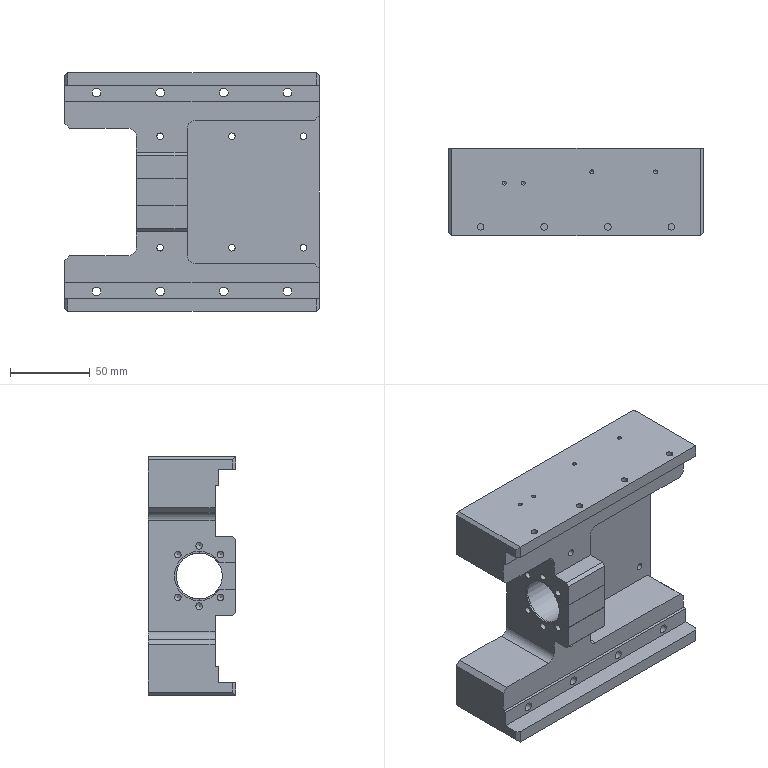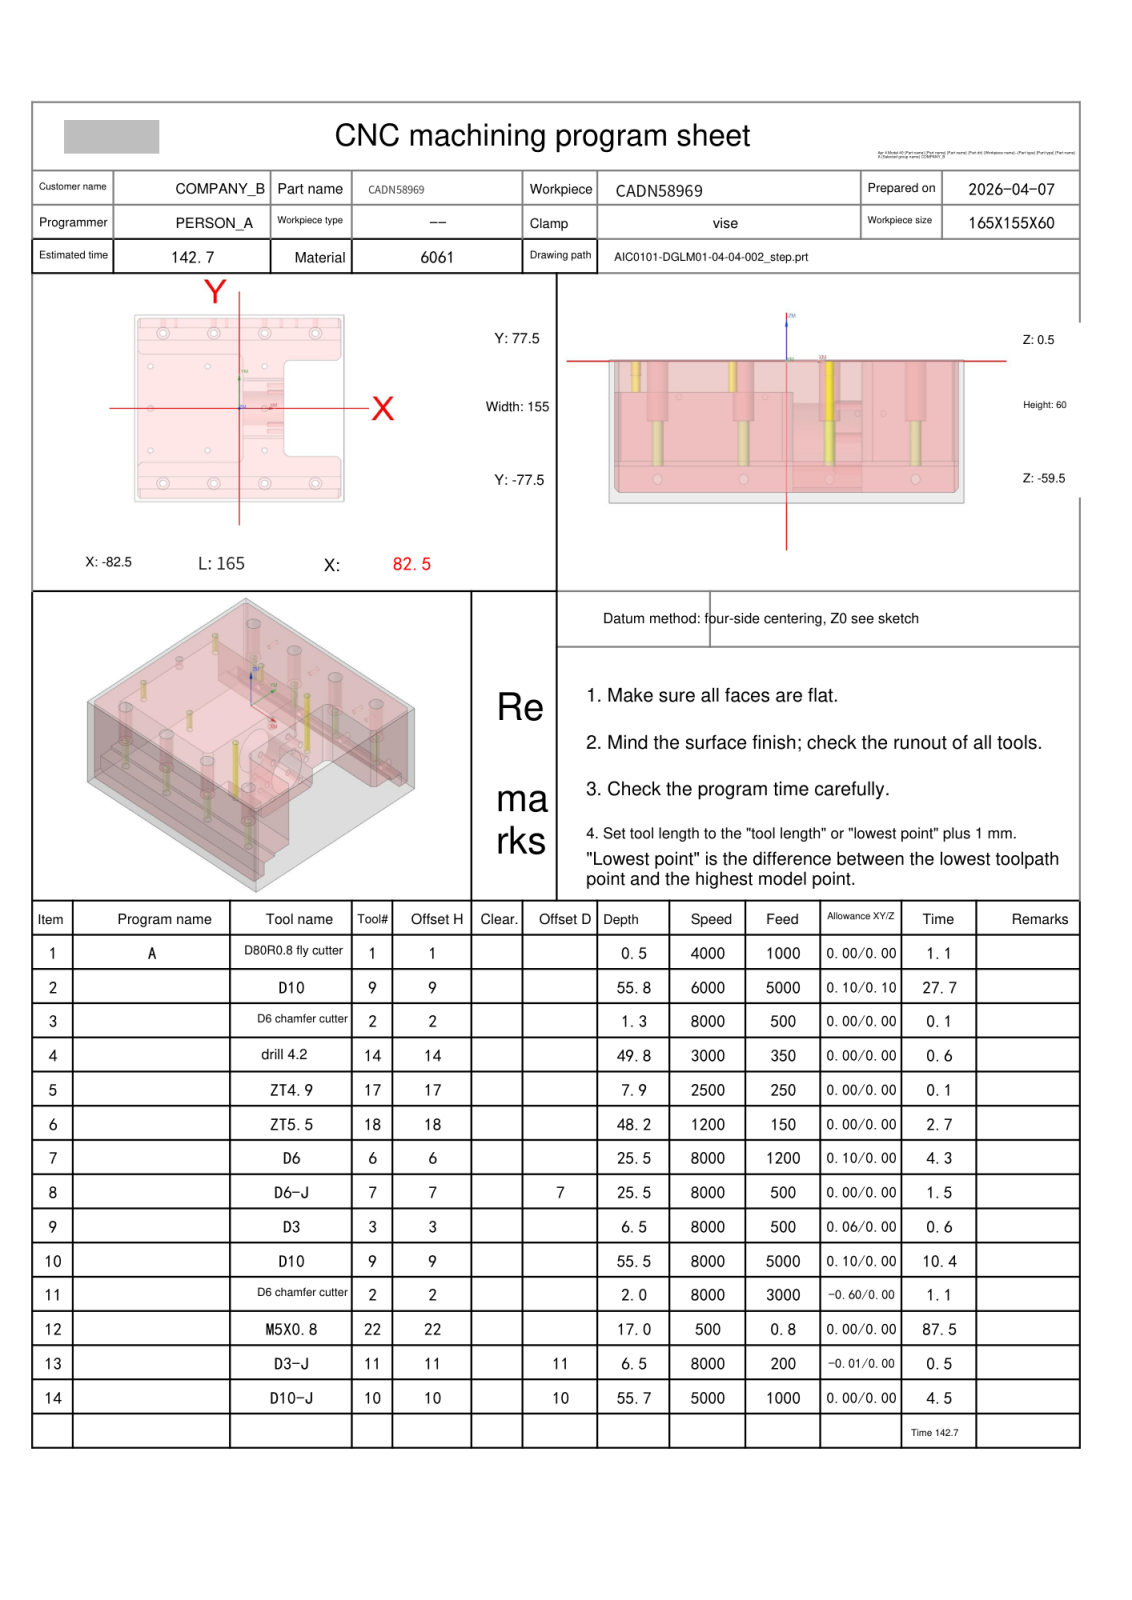NC program | NX | posted by the shop | part box 160 x 55 x 150 mm
Lines 45 to 1090 of 15707:
N2 T09 M06
(D10  D=10. R=0. H=09 ce=0.10 di=0.10)
G00 G90 G54 X94.5 Y.734 M03 S6000
G43 H09 Z10.5
M08
Z.702
G01 Z-.498 F5000.
G02 X89.333 Y-1.543 I-5.167 J4.722
X87.5 Y-1.299 I0.0 J7.
G03 X83.279 Y-.395 I-10.5 J-38.701
G02 X82.944 Y0.0 I.065 J.395
X83.279 Y.395 I.4 J0.0
G03 X86.743 Y1.102 I-6.279 J39.605
X87.5 Y2.071 I-.243 J.97
G01 Y7.652
G03 X86.8 Y8.352 I-.7 J0.0
X86.597 Y8.322 I0.0 J-.7
G02 X77. Y6.9 I-9.597 J31.678
G01 X69.096
G03 X68.1 Y5.904 I.004 J-1.
G01 Y-2.564
X68.078 Y-2.653
X68.156 Y-2.699
X68.29 Y-2.831
G02 X68.377 Y-3.015 I-.21 J-.213
G03 X70.866 Y-5.276 I2.489 J.238
X71.779 Y-5.104 I0.0 J2.5
G01 X81.091 Y-1.451
G03 X82.679 Y.876 I-.913 J2.327
X80.179 Y3.376 I-2.5 J0.0
X79.266 Y3.204 I0.0 J-2.5
G01 X69.953 Y-.449
G03 X68.374 Y-2.575 I.913 J-2.327
G01 X68.393 Y-2.656
X68.318 Y-2.694
X68.191 Y-2.819
G03 X68.1 Y-3.037 I.215 J-.218
G01 Y-5.904
G03 X69.096 Y-6.9 I1. J.004
G01 X77.
G02 X86.796 Y-8.383 I0.0 J-33.1
X87.5 Y-9.338 I-.296 J-.955
G01 Y-15.203
G02 X86.9 Y-15.803 I-.6 J0.0
X86.678 Y-15.761 I0.0 J.6
G03 X77. Y-13.9 I-9.678 J-24.239
G01 X62.097
G02 X61.1 Y-12.903 I.003 J1.
G01 Y12.903
G02 X62.097 Y13.9 I1. J-.003
G01 X77.
G03 X86.879 Y15.842 I0.0 J26.1
X87.5 Y16.767 I-.379 J.925
G01 Y23.143
G03 X87. Y23.643 I-.5 J0.0
X86.745 Y23.573 I0.0 J-.5
G02 X77. Y20.9 I-9.745 J16.427
G01 X55.097
G03 X54.1 Y19.903 I.003 J-1.
G01 Y-19.903
G03 X55.097 Y-20.9 I1. J.003
G01 X77.
G02 X87.025 Y-23.743 I0.0 J-19.1
X87.5 Y-24.593 I-.525 J-.851
G01 Y-32.423
G02 X87.1 Y-32.822 I-.4 J0.0
X86.817 Y-32.705 I0.0 J.4
G01 X85.556 Y-31.444
G03 X77. Y-27.9 I-8.556 J-8.556
G01 X48.098
G02 X47.1 Y-26.902 I.002 J1.
G01 Y26.902
G02 X48.098 Y27.9 I1. J-.002
G01 X77.
G03 X85.556 Y31.444 I0.0 J12.1
G01 X86.903 Y32.791
G03 X87.195 Y33.498 I-.707 J.707
X87.011 Y34.077 I-1. J0.0
G01 X84.072 Y38.21
G03 X83.257 Y38.631 I-.815 J-.579
X82.55 Y38.338 I0.0 J-1.
G01 X80.606 Y36.394
G02 X77. Y34.9 I-3.606 J3.606
G01 X40.1
Y-34.9
X77.
G02 X80.606 Y-36.394 I0.0 J-5.1
G01 X83.606 Y-39.394
G02 X85.1 Y-43. I-3.606 J-3.606
G01 Y-73.001
G02 X83.606 Y-76.606 I-5.1 J.001
G01 X81.606 Y-78.606
G02 X78. Y-80.1 I-3.606 J3.606
G01 X-78.
G02 X-81.606 Y-78.606 I0.0 J5.1
G01 X-83.606 Y-76.606
G02 X-85.1 Y-73.001 I3.606 J3.606
G01 Y73.001
G02 X-83.606 Y76.606 I5.1 J-.001
G01 X-81.606 Y78.606
G02 X-78. Y80.1 I3.606 J-3.606
G01 X78.
G02 X81.606 Y78.606 I0.0 J-5.1
G01 X83.606 Y76.606
G02 X85.1 Y73.001 I-3.606 J-3.606
G01 Y43.
G02 X83.606 Y39.394 I-5.1 J0.0
G01 X80.606 Y36.394
G02 X78.72 Y35.199 I-3.606 J3.606
X78.242 Y35.054 I-1.72 J4.801
G03 X72.947 Y28.264 I1.705 J-6.789
X73.158 Y26.559 I7. J0.0
G01 Z.702
G00 Z3.
G01 X94.5 Y.734 F6000.
G00 Z.204
G01 Z-.996 F5000.
G02 X89.333 Y-1.543 I-5.167 J4.722
X87.5 Y-1.299 I0.0 J7.
G03 X83.279 Y-.395 I-10.5 J-38.701
G02 X82.944 Y0.0 I.065 J.395
X83.279 Y.395 I.4 J0.0
G03 X86.743 Y1.102 I-6.279 J39.605
X87.5 Y2.071 I-.243 J.97
G01 Y7.652
G03 X86.8 Y8.352 I-.7 J0.0
X86.597 Y8.322 I0.0 J-.7
G02 X77. Y6.9 I-9.597 J31.678
G01 X69.096
G03 X68.1 Y5.904 I.004 J-1.
G01 Y2.988
X68.078 Y2.9
X68.156 Y2.854
X68.29 Y2.722
G02 X68.377 Y2.538 I-.21 J-.213
G03 X69.953 Y.449 I2.489 J.238
G01 X79.266 Y-3.204
G03 X80.179 Y-3.376 I.913 J2.327
X82.679 Y-.876 I0.0 J2.5
X81.091 Y1.451 I-2.5 J0.0
G01 X71.779 Y5.104
G03 X70.866 Y5.276 I-.913 J-2.327
X68.374 Y2.978 I0.0 J-2.5
G01 X68.393 Y2.897
X68.318 Y2.859
X68.191 Y2.734
G03 X68.1 Y2.515 I.215 J-.218
G01 Y-5.904
G03 X69.096 Y-6.9 I1. J.004
G01 X77.
G02 X86.796 Y-8.383 I0.0 J-33.1
X87.5 Y-9.338 I-.296 J-.955
G01 Y-15.203
G02 X86.9 Y-15.803 I-.6 J0.0
X86.678 Y-15.761 I0.0 J.6
G03 X77. Y-13.9 I-9.678 J-24.239
G01 X62.097
G02 X61.1 Y-12.903 I.003 J1.
G01 Y12.903
G02 X62.097 Y13.9 I1. J-.003
G01 X77.
G03 X86.879 Y15.842 I0.0 J26.1
X87.5 Y16.767 I-.379 J.925
G01 Y23.143
G03 X87. Y23.643 I-.5 J0.0
X86.745 Y23.573 I0.0 J-.5
G02 X77. Y20.9 I-9.745 J16.427
G01 X55.097
G03 X54.1 Y19.903 I.003 J-1.
G01 Y-19.903
G03 X55.097 Y-20.9 I1. J.003
G01 X77.
G02 X87.025 Y-23.742 I0.0 J-19.1
X87.5 Y-24.593 I-.525 J-.851
G01 Y-32.423
G02 X87.1 Y-32.822 I-.4 J0.0
X86.817 Y-32.705 I0.0 J.4
G01 X85.556 Y-31.444
G03 X77. Y-27.9 I-8.556 J-8.556
G01 X48.098
G02 X47.1 Y-26.902 I.002 J1.
G01 Y26.902
G02 X48.098 Y27.9 I1. J-.002
G01 X77.
G03 X85.556 Y31.444 I0.0 J12.1
G01 X86.903 Y32.791
G03 X87.195 Y33.498 I-.707 J.707
X87.011 Y34.077 I-1. J0.0
G01 X84.072 Y38.21
G03 X83.257 Y38.631 I-.815 J-.579
X82.55 Y38.338 I0.0 J-1.
G01 X80.606 Y36.394
G02 X77. Y34.9 I-3.606 J3.606
G01 X40.1
Y-34.9
X77.
G02 X80.606 Y-36.394 I0.0 J-5.1
G01 X83.606 Y-39.394
G02 X85.1 Y-43. I-3.606 J-3.606
G01 Y-73.001
G02 X83.606 Y-76.606 I-5.1 J.001
G01 X81.606 Y-78.606
G02 X78. Y-80.1 I-3.606 J3.606
G01 X-78.
G02 X-81.606 Y-78.606 I0.0 J5.1
G01 X-83.606 Y-76.606
G02 X-85.1 Y-73.001 I3.606 J3.606
G01 Y73.001
G02 X-83.606 Y76.606 I5.1 J-.001
G01 X-81.606 Y78.606
G02 X-78. Y80.1 I3.606 J-3.606
G01 X78.
G02 X81.606 Y78.606 I0.0 J-5.1
G01 X83.606 Y76.606
G02 X85.1 Y73.001 I-3.606 J-3.606
G01 Y43.
G02 X83.606 Y39.394 I-5.1 J0.0
G01 X80.606 Y36.394
G02 X78.72 Y35.199 I-3.606 J3.606
X78.242 Y35.054 I-1.72 J4.801
G03 X72.947 Y28.264 I1.705 J-6.789
X73.158 Y26.559 I7. J0.0
G01 Z.204
G00 Z2.502
G01 X94.5 Y.734 F6000.
G00 Z-.295
G01 Z-1.495 F5000.
G02 X89.333 Y-1.543 I-5.167 J4.722
X87.5 Y-1.299 I0.0 J7.
G03 X83.279 Y-.395 I-10.5 J-38.701
G02 X82.944 Y0.0 I.065 J.395
X83.279 Y.395 I.4 J0.0
G03 X86.743 Y1.102 I-6.279 J39.605
X87.5 Y2.071 I-.243 J.97
G01 Y7.652
G03 X86.8 Y8.352 I-.7 J0.0
X86.597 Y8.322 I0.0 J-.7
G02 X77. Y6.9 I-9.597 J31.678
G01 X69.097
G03 X68.1 Y5.903 I.003 J-1.
G01 Y2.988
X68.078 Y2.9
X68.156 Y2.854
X68.29 Y2.722
G02 X68.377 Y2.538 I-.21 J-.213
G03 X69.953 Y.449 I2.489 J.238
G01 X79.266 Y-3.204
G03 X80.179 Y-3.376 I.913 J2.327
X82.679 Y-.876 I0.0 J2.5
X81.091 Y1.451 I-2.5 J0.0
G01 X71.779 Y5.104
G03 X70.866 Y5.276 I-.913 J-2.327
X68.374 Y2.978 I0.0 J-2.5
G01 X68.393 Y2.897
X68.318 Y2.859
X68.191 Y2.734
G03 X68.1 Y2.515 I.215 J-.218
G01 Y-5.903
G03 X69.097 Y-6.9 I1. J.003
G01 X77.
G02 X86.796 Y-8.383 I0.0 J-33.1
X87.5 Y-9.338 I-.296 J-.955
G01 Y-15.203
G02 X86.9 Y-15.803 I-.6 J0.0
X86.678 Y-15.761 I0.0 J.6
G03 X77. Y-13.9 I-9.678 J-24.239
G01 X62.097
G02 X61.1 Y-12.903 I.003 J1.
G01 Y12.903
G02 X62.097 Y13.9 I1. J-.003
G01 X77.
G03 X86.879 Y15.842 I0.0 J26.1
X87.5 Y16.767 I-.379 J.925
G01 Y23.143
G03 X87. Y23.643 I-.5 J0.0
X86.745 Y23.573 I0.0 J-.5
G02 X77. Y20.9 I-9.745 J16.427
G01 X55.098
G03 X54.1 Y19.902 I.002 J-1.
G01 Y-19.902
G03 X55.098 Y-20.9 I1. J.002
G01 X77.
G02 X87.025 Y-23.743 I0.0 J-19.1
X87.5 Y-24.593 I-.525 J-.851
G01 Y-32.423
G02 X87.1 Y-32.822 I-.4 J0.0
X86.817 Y-32.705 I0.0 J.4
G01 X85.556 Y-31.444
G03 X77. Y-27.9 I-8.556 J-8.556
G01 X48.099
G02 X47.1 Y-26.901 I.001 J1.
G01 Y26.901
G02 X48.099 Y27.9 I1. J-.001
G01 X77.
G03 X85.556 Y31.444 I0.0 J12.1
G01 X86.903 Y32.791
G03 X87.195 Y33.498 I-.707 J.707
X87.011 Y34.077 I-1. J0.0
G01 X84.072 Y38.21
G03 X83.257 Y38.631 I-.815 J-.579
X82.55 Y38.338 I0.0 J-1.
G01 X80.606 Y36.394
G02 X77. Y34.9 I-3.606 J3.606
G01 X40.1
Y-34.9
X77.
G02 X80.606 Y-36.394 I0.0 J-5.1
G01 X83.606 Y-39.394
G02 X85.1 Y-43. I-3.606 J-3.606
G01 Y-73.
G02 X83.606 Y-76.606 I-5.1 J0.0
G01 X81.606 Y-78.606
G02 X78. Y-80.1 I-3.606 J3.606
G01 X-78.
G02 X-81.606 Y-78.606 I0.0 J5.1
G01 X-83.606 Y-76.606
G02 X-85.1 Y-73. I3.606 J3.606
G01 Y73.
G02 X-83.606 Y76.606 I5.1 J0.0
G01 X-81.606 Y78.606
G02 X-78. Y80.1 I3.606 J-3.606
G01 X78.
G02 X81.606 Y78.606 I0.0 J-5.1
G01 X83.606 Y76.606
G02 X85.1 Y73. I-3.606 J-3.606
G01 Y43.
G02 X83.606 Y39.394 I-5.1 J0.0
G01 X80.606 Y36.394
G02 X78.72 Y35.199 I-3.606 J3.606
X78.242 Y35.054 I-1.72 J4.801
G03 X72.947 Y28.264 I1.705 J-6.789
X73.158 Y26.559 I7. J0.0
G01 Z-.295
G00 Z2.004
G01 X94.5 Y.734 F6000.
G00 Z-.793
G01 Z-1.993 F5000.
G02 X89.333 Y-1.543 I-5.167 J4.722
X87.5 Y-1.299 I0.0 J7.
G03 X83.279 Y-.395 I-10.5 J-38.701
G02 X82.944 Y0.0 I.065 J.395
X83.279 Y.395 I.4 J0.0
G03 X86.743 Y1.102 I-6.279 J39.605
X87.5 Y2.071 I-.243 J.97
G01 Y7.652
G03 X86.8 Y8.352 I-.7 J0.0
X86.597 Y8.322 I0.0 J-.7
G02 X77. Y6.9 I-9.597 J31.678
G01 X69.096
G03 X68.1 Y5.904 I.004 J-1.
G01 Y-2.564
X68.078 Y-2.653
X68.156 Y-2.699
X68.29 Y-2.831
G02 X68.377 Y-3.015 I-.21 J-.213
G03 X70.866 Y-5.276 I2.489 J.238
X71.779 Y-5.104 I0.0 J2.5
G01 X81.091 Y-1.451
G03 X82.679 Y.876 I-.913 J2.327
X80.179 Y3.376 I-2.5 J0.0
X79.266 Y3.204 I0.0 J-2.5
G01 X69.953 Y-.449
G03 X68.374 Y-2.575 I.913 J-2.327
G01 X68.393 Y-2.656
X68.318 Y-2.694
X68.191 Y-2.819
G03 X68.1 Y-3.037 I.215 J-.218
G01 Y-5.904
G03 X69.096 Y-6.9 I1. J.004
G01 X77.
G02 X86.796 Y-8.383 I0.0 J-33.1
X87.5 Y-9.338 I-.296 J-.955
G01 Y-15.203
G02 X86.9 Y-15.803 I-.6 J0.0
X86.678 Y-15.761 I0.0 J.6
G03 X77. Y-13.9 I-9.678 J-24.239
G01 X62.097
G02 X61.1 Y-12.903 I.003 J1.
G01 Y12.903
G02 X62.097 Y13.9 I1. J-.003
G01 X77.
G03 X86.879 Y15.842 I0.0 J26.1
X87.5 Y16.767 I-.379 J.925
G01 Y23.143
G03 X87. Y23.643 I-.5 J0.0
X86.745 Y23.573 I0.0 J-.5
G02 X77. Y20.9 I-9.745 J16.427
G01 X55.098
G03 X54.1 Y19.902 I.002 J-1.
G01 Y-19.902
G03 X55.098 Y-20.9 I1. J.002
G01 X77.
G02 X87.025 Y-23.743 I0.0 J-19.1
X87.5 Y-24.593 I-.525 J-.851
G01 Y-32.423
G02 X87.1 Y-32.822 I-.4 J0.0
X86.817 Y-32.705 I0.0 J.4
G01 X85.556 Y-31.444
G03 X77. Y-27.9 I-8.556 J-8.556
G01 X48.099
G02 X47.1 Y-26.901 I.001 J1.
G01 Y26.901
G02 X48.099 Y27.9 I1. J-.001
G01 X77.
G03 X85.556 Y31.444 I0.0 J12.1
G01 X86.903 Y32.791
G03 X87.195 Y33.498 I-.707 J.707
X87.011 Y34.077 I-1. J0.0
G01 X84.072 Y38.21
G03 X83.257 Y38.631 I-.815 J-.579
X82.55 Y38.338 I0.0 J-1.
G01 X80.606 Y36.394
G02 X77. Y34.9 I-3.606 J3.606
G01 X40.1
Y-34.9
X77.
G02 X80.606 Y-36.394 I0.0 J-5.1
G01 X83.606 Y-39.394
G02 X85.1 Y-43. I-3.606 J-3.606
G01 Y-73.
G02 X83.606 Y-76.606 I-5.1 J0.0
G01 X81.606 Y-78.606
G02 X78. Y-80.1 I-3.606 J3.606
G01 X-78.
G02 X-81.606 Y-78.606 I0.0 J5.1
G01 X-83.606 Y-76.606
G02 X-85.1 Y-73. I3.606 J3.606
G01 Y73.
G02 X-83.606 Y76.606 I5.1 J0.0
G01 X-81.606 Y78.606
G02 X-78. Y80.1 I3.606 J-3.606
G01 X78.
G02 X81.606 Y78.606 I0.0 J-5.1
G01 X83.606 Y76.606
G02 X85.1 Y73. I-3.606 J-3.606
G01 Y43.
G02 X83.606 Y39.394 I-5.1 J0.0
G01 X80.606 Y36.394
G02 X78.72 Y35.199 I-3.606 J3.606
X78.242 Y35.054 I-1.72 J4.801
G03 X72.947 Y28.264 I1.705 J-6.789
X73.158 Y26.559 I7. J0.0
G01 Z-.793
G00 Z1.505
G01 X94.5 Y.734 F6000.
G00 Z-1.291
G01 Z-2.491 F5000.
G02 X89.333 Y-1.543 I-5.167 J4.722
X87.5 Y-1.299 I0.0 J7.
G03 X83.279 Y-.395 I-10.5 J-38.701
G02 X82.944 Y0.0 I.065 J.395
X83.279 Y.395 I.4 J0.0
G03 X86.743 Y1.102 I-6.279 J39.605
X87.5 Y2.071 I-.243 J.97
G01 Y7.652
G03 X86.8 Y8.352 I-.7 J0.0
X86.597 Y8.322 I0.0 J-.7
G02 X77. Y6.9 I-9.597 J31.678
G01 X69.097
G03 X68.1 Y5.903 I.003 J-1.
G01 Y2.988
X68.078 Y2.9
X68.156 Y2.854
X68.29 Y2.722
G02 X68.377 Y2.538 I-.21 J-.213
G03 X69.953 Y.449 I2.489 J.238
G01 X79.266 Y-3.204
G03 X80.179 Y-3.376 I.913 J2.327
X82.679 Y-.876 I0.0 J2.5
X81.091 Y1.451 I-2.5 J0.0
G01 X71.779 Y5.104
G03 X70.866 Y5.276 I-.913 J-2.327
X68.374 Y2.978 I0.0 J-2.5
G01 X68.393 Y2.897
X68.318 Y2.859
X68.191 Y2.734
G03 X68.1 Y2.515 I.215 J-.218
G01 Y-5.903
G03 X69.097 Y-6.9 I1. J.003
G01 X77.
G02 X86.796 Y-8.383 I0.0 J-33.1
X87.5 Y-9.338 I-.296 J-.955
G01 Y-15.203
G02 X86.9 Y-15.803 I-.6 J0.0
X86.678 Y-15.761 I0.0 J.6
G03 X77. Y-13.9 I-9.678 J-24.239
G01 X62.097
G02 X61.1 Y-12.903 I.003 J1.
G01 Y12.903
G02 X62.097 Y13.9 I1. J-.003
G01 X77.
G03 X86.879 Y15.842 I0.0 J26.1
X87.5 Y16.767 I-.379 J.925
G01 Y23.143
G03 X87. Y23.643 I-.5 J0.0
X86.745 Y23.573 I0.0 J-.5
G02 X77. Y20.9 I-9.745 J16.427
G01 X55.098
G03 X54.1 Y19.902 I.002 J-1.
G01 Y-19.902
G03 X55.098 Y-20.9 I1. J.002
G01 X77.
G02 X87.025 Y-23.743 I0.0 J-19.1
X87.5 Y-24.593 I-.525 J-.851
G01 Y-32.423
G02 X87.1 Y-32.822 I-.4 J0.0
X86.817 Y-32.705 I0.0 J.4
G01 X85.556 Y-31.444
G03 X77. Y-27.9 I-8.556 J-8.556
G01 X48.099
G02 X47.1 Y-26.901 I.001 J1.
G01 Y26.901
G02 X48.099 Y27.9 I1. J-.001
G01 X77.
G03 X85.556 Y31.444 I0.0 J12.1
G01 X86.903 Y32.791
G03 X87.195 Y33.498 I-.707 J.707
X87.011 Y34.077 I-1. J0.0
G01 X84.072 Y38.21
G03 X83.257 Y38.631 I-.815 J-.579
X82.55 Y38.338 I0.0 J-1.
G01 X80.606 Y36.394
G02 X77. Y34.9 I-3.606 J3.606
G01 X40.1
Y-34.9
X77.
G02 X80.606 Y-36.394 I0.0 J-5.1
G01 X83.606 Y-39.394
G02 X85.1 Y-43. I-3.606 J-3.606
G01 Y-73.
G02 X83.606 Y-76.606 I-5.1 J0.0
G01 X81.606 Y-78.606
G02 X78. Y-80.1 I-3.606 J3.606
G01 X-78.
G02 X-81.606 Y-78.606 I0.0 J5.1
G01 X-83.606 Y-76.606
G02 X-85.1 Y-73. I3.606 J3.606
G01 Y73.
G02 X-83.606 Y76.606 I5.1 J0.0
G01 X-81.606 Y78.606
G02 X-78. Y80.1 I3.606 J-3.606
G01 X78.
G02 X81.606 Y78.606 I0.0 J-5.1
G01 X83.606 Y76.606
G02 X85.1 Y73. I-3.606 J-3.606
G01 Y43.
G02 X83.606 Y39.394 I-5.1 J0.0
G01 X80.606 Y36.394
G02 X78.72 Y35.199 I-3.606 J3.606
X78.242 Y35.054 I-1.72 J4.801
G03 X72.947 Y28.264 I1.705 J-6.789
X73.158 Y26.559 I7. J0.0
G01 Z-1.291
G00 Z1.007
G01 X94.5 Y.734 F6000.
G00 Z-1.789
G01 Z-2.989 F5000.
G02 X89.333 Y-1.543 I-5.167 J4.722
X87.5 Y-1.299 I0.0 J7.
G03 X83.279 Y-.395 I-10.5 J-38.701
G02 X82.944 Y0.0 I.065 J.395
X83.279 Y.395 I.4 J0.0
G03 X86.743 Y1.102 I-6.279 J39.605
X87.5 Y2.071 I-.243 J.97
G01 Y7.652
G03 X86.8 Y8.352 I-.7 J0.0
X86.597 Y8.322 I0.0 J-.7
G02 X77. Y6.9 I-9.597 J31.678
G01 X69.096
G03 X68.1 Y5.904 I.004 J-1.
G01 Y-2.564
X68.078 Y-2.653
X68.156 Y-2.699
X68.29 Y-2.831
G02 X68.377 Y-3.015 I-.21 J-.213
G03 X70.866 Y-5.276 I2.489 J.238
X71.779 Y-5.104 I0.0 J2.5
G01 X81.091 Y-1.451
G03 X82.679 Y.876 I-.913 J2.327
X80.179 Y3.376 I-2.5 J0.0
X79.266 Y3.204 I0.0 J-2.5
G01 X69.953 Y-.449
G03 X68.374 Y-2.575 I.913 J-2.327
G01 X68.393 Y-2.656
X68.318 Y-2.694
X68.191 Y-2.819
G03 X68.1 Y-3.037 I.215 J-.218
G01 Y-5.904
G03 X69.096 Y-6.9 I1. J.004
G01 X77.
G02 X86.796 Y-8.383 I0.0 J-33.1
X87.5 Y-9.338 I-.296 J-.955
G01 Y-15.203
G02 X86.9 Y-15.803 I-.6 J0.0
X86.678 Y-15.761 I0.0 J.6
G03 X77. Y-13.9 I-9.678 J-24.239
G01 X62.097
G02 X61.1 Y-12.903 I.003 J1.
G01 Y12.903
G02 X62.097 Y13.9 I1. J-.003
G01 X77.
G03 X86.879 Y15.842 I0.0 J26.1
X87.5 Y16.767 I-.379 J.925
G01 Y23.143
G03 X87. Y23.643 I-.5 J0.0
X86.745 Y23.573 I0.0 J-.5
G02 X77. Y20.9 I-9.745 J16.427
G01 X55.098
G03 X54.1 Y19.902 I.002 J-1.
G01 Y-19.902
G03 X55.098 Y-20.9 I1. J.002
G01 X77.
G02 X87.025 Y-23.743 I0.0 J-19.1
X87.5 Y-24.593 I-.525 J-.851
G01 Y-32.423
G02 X87.1 Y-32.822 I-.4 J0.0
X86.817 Y-32.705 I0.0 J.4
G01 X85.556 Y-31.444
G03 X77. Y-27.9 I-8.556 J-8.556
G01 X48.099
G02 X47.1 Y-26.901 I.001 J1.
G01 Y26.901
G02 X48.099 Y27.9 I1. J-.001
G01 X77.
G03 X85.556 Y31.444 I0.0 J12.1
G01 X86.903 Y32.791
G03 X87.195 Y33.498 I-.707 J.707
X87.011 Y34.077 I-1. J0.0
G01 X84.072 Y38.21
G03 X83.257 Y38.631 I-.815 J-.579
X82.55 Y38.338 I0.0 J-1.
G01 X80.606 Y36.394
G02 X77. Y34.9 I-3.606 J3.606
G01 X40.1
Y-34.9
X77.
G02 X80.606 Y-36.394 I0.0 J-5.1
G01 X83.606 Y-39.394
G02 X85.1 Y-43. I-3.606 J-3.606
G01 Y-73.
G02 X83.606 Y-76.606 I-5.1 J0.0
G01 X81.606 Y-78.606
G02 X78. Y-80.1 I-3.606 J3.606
G01 X-78.
G02 X-81.606 Y-78.606 I0.0 J5.1
G01 X-83.606 Y-76.606
G02 X-85.1 Y-73. I3.606 J3.606
G01 Y73.
G02 X-83.606 Y76.606 I5.1 J0.0
G01 X-81.606 Y78.606
G02 X-78. Y80.1 I3.606 J-3.606
G01 X78.
G02 X81.606 Y78.606 I0.0 J-5.1
G01 X83.606 Y76.606
G02 X85.1 Y73. I-3.606 J-3.606
G01 Y43.
G02 X83.606 Y39.394 I-5.1 J0.0
G01 X80.606 Y36.394
G02 X78.72 Y35.199 I-3.606 J3.606
X78.242 Y35.054 I-1.72 J4.801
G03 X72.947 Y28.264 I1.705 J-6.789
X73.158 Y26.559 I7. J0.0
G01 Z-1.789
G00 Z.509
G01 X94.5 Y.734 F6000.
G00 Z-2.287
G01 Z-3.487 F5000.
G02 X89.333 Y-1.543 I-5.167 J4.722
X87.5 Y-1.299 I0.0 J7.
G03 X83.279 Y-.395 I-10.5 J-38.701
G02 X82.944 Y0.0 I.065 J.395
X83.279 Y.395 I.4 J0.0
G03 X86.743 Y1.102 I-6.279 J39.605
X87.5 Y2.071 I-.243 J.97
G01 Y7.652
G03 X86.8 Y8.352 I-.7 J0.0
X86.597 Y8.322 I0.0 J-.7
G02 X77. Y6.9 I-9.597 J31.678
G01 X69.097
G03 X68.1 Y5.903 I.003 J-1.
G01 Y2.988
X68.078 Y2.9
X68.156 Y2.854
X68.29 Y2.722
G02 X68.377 Y2.538 I-.21 J-.213
G03 X69.953 Y.449 I2.489 J.238
G01 X79.266 Y-3.204
G03 X80.179 Y-3.376 I.913 J2.327
X82.679 Y-.876 I0.0 J2.5
X81.091 Y1.451 I-2.5 J0.0
G01 X71.779 Y5.104
G03 X70.866 Y5.276 I-.913 J-2.327
X68.374 Y2.978 I0.0 J-2.5
G01 X68.393 Y2.897
X68.318 Y2.859
X68.191 Y2.734
G03 X68.1 Y2.515 I.215 J-.218
G01 Y-5.903
G03 X69.097 Y-6.9 I1. J.003
G01 X77.
G02 X86.796 Y-8.383 I0.0 J-33.1
X87.5 Y-9.338 I-.296 J-.955
G01 Y-15.203
G02 X86.9 Y-15.803 I-.6 J0.0
X86.678 Y-15.761 I0.0 J.6
G03 X77. Y-13.9 I-9.678 J-24.239
G01 X62.097
G02 X61.1 Y-12.903 I.003 J1.
G01 Y12.903
G02 X62.097 Y13.9 I1. J-.003
G01 X77.
G03 X86.879 Y15.842 I0.0 J26.1
X87.5 Y16.767 I-.379 J.925
G01 Y23.143
G03 X87. Y23.643 I-.5 J0.0
X86.745 Y23.573 I0.0 J-.5
G02 X77. Y20.9 I-9.745 J16.427
G01 X55.098
G03 X54.1 Y19.902 I.002 J-1.
G01 Y-19.902
G03 X55.098 Y-20.9 I1. J.002
G01 X77.
G02 X87.025 Y-23.743 I0.0 J-19.1
X87.5 Y-24.593 I-.525 J-.851
G01 Y-32.423
G02 X87.1 Y-32.822 I-.4 J0.0
X86.817 Y-32.705 I0.0 J.4
G01 X85.556 Y-31.444
G03 X77. Y-27.9 I-8.556 J-8.556
G01 X48.099
G02 X47.1 Y-26.901 I.001 J1.
G01 Y26.901
G02 X48.099 Y27.9 I1. J-.001
G01 X77.
G03 X85.556 Y31.444 I0.0 J12.1
G01 X86.903 Y32.791
G03 X87.195 Y33.498 I-.707 J.707
X87.011 Y34.077 I-1. J0.0
G01 X84.072 Y38.21
G03 X83.257 Y38.631 I-.815 J-.579
X82.55 Y38.338 I0.0 J-1.
G01 X80.606 Y36.394
G02 X77. Y34.9 I-3.606 J3.606
G01 X40.1
Y-34.9
X77.
G02 X80.606 Y-36.394 I0.0 J-5.1
G01 X83.606 Y-39.394
G02 X85.1 Y-43. I-3.606 J-3.606
G01 Y-73.
G02 X83.606 Y-76.606 I-5.1 J0.0
G01 X81.606 Y-78.606
G02 X78. Y-80.1 I-3.606 J3.606
G01 X-78.
G02 X-81.606 Y-78.606 I0.0 J5.1
G01 X-83.606 Y-76.606
G02 X-85.1 Y-73. I3.606 J3.606
G01 Y73.
G02 X-83.606 Y76.606 I5.1 J0.0
G01 X-81.606 Y78.606
G02 X-78. Y80.1 I3.606 J-3.606
G01 X78.
G02 X81.606 Y78.606 I0.0 J-5.1
G01 X83.606 Y76.606
G02 X85.1 Y73. I-3.606 J-3.606
G01 Y43.
G02 X83.606 Y39.394 I-5.1 J0.0
G01 X80.606 Y36.394
G02 X78.72 Y35.199 I-3.606 J3.606
X78.242 Y35.054 I-1.72 J4.801
G03 X72.947 Y28.264 I1.705 J-6.789
X73.158 Y26.559 I7. J0.0
G01 Z-2.287
G00 Z.011
G01 X94.5 Y.734 F6000.
G00 Z-2.786
G01 Z-3.986 F5000.
G02 X89.333 Y-1.543 I-5.167 J4.722
X87.5 Y-1.299 I0.0 J7.
G03 X83.279 Y-.395 I-10.5 J-38.701
G02 X82.944 Y0.0 I.065 J.395
X83.279 Y.395 I.4 J0.0
G03 X86.743 Y1.102 I-6.279 J39.605
X87.5 Y2.071 I-.243 J.97
G01 Y7.652
G03 X86.8 Y8.352 I-.7 J0.0
X86.597 Y8.322 I0.0 J-.7
G02 X77. Y6.9 I-9.597 J31.678
G01 X69.096
G03 X68.1 Y5.904 I.004 J-1.
G01 Y-2.564
X68.078 Y-2.653
X68.156 Y-2.699
X68.29 Y-2.831
G02 X68.377 Y-3.015 I-.21 J-.213
G03 X70.866 Y-5.276 I2.489 J.238
X71.779 Y-5.104 I0.0 J2.5
G01 X81.091 Y-1.451
G03 X82.679 Y.876 I-.913 J2.327
X80.179 Y3.376 I-2.5 J0.0
X79.266 Y3.204 I0.0 J-2.5
G01 X69.953 Y-.449
G03 X68.374 Y-2.575 I.913 J-2.327
G01 X68.393 Y-2.656
X68.318 Y-2.694
X68.191 Y-2.819
G03 X68.1 Y-3.037 I.215 J-.218
G01 Y-5.904
G03 X69.096 Y-6.9 I1. J.004
G01 X77.
G02 X86.796 Y-8.383 I0.0 J-33.1
X87.5 Y-9.338 I-.296 J-.955
G01 Y-15.203
G02 X86.9 Y-15.803 I-.6 J0.0
X86.678 Y-15.761 I0.0 J.6
G03 X77. Y-13.9 I-9.678 J-24.239
G01 X62.097
G02 X61.1 Y-12.903 I.003 J1.
G01 Y12.903
G02 X62.097 Y13.9 I1. J-.003
G01 X77.
G03 X86.879 Y15.842 I0.0 J26.1
X87.5 Y16.767 I-.379 J.925
G01 Y23.143
G03 X87. Y23.643 I-.5 J0.0
X86.745 Y23.573 I0.0 J-.5
G02 X77. Y20.9 I-9.745 J16.427
G01 X55.098
G03 X54.1 Y19.902 I.002 J-1.
G01 Y-19.902
G03 X55.098 Y-20.9 I1. J.002
G01 X77.
G02 X87.025 Y-23.743 I0.0 J-19.1
X87.5 Y-24.593 I-.525 J-.851
G01 Y-32.423
G02 X87.1 Y-32.822 I-.4 J0.0
X86.817 Y-32.705 I0.0 J.4
G01 X85.556 Y-31.444
G03 X77. Y-27.9 I-8.556 J-8.556
G01 X48.099
G02 X47.1 Y-26.901 I.001 J1.
G01 Y26.901
G02 X48.099 Y27.9 I1. J-.001
G01 X77.
G03 X85.556 Y31.444 I0.0 J12.1
G01 X86.903 Y32.791
G03 X87.195 Y33.498 I-.707 J.707
X87.011 Y34.077 I-1. J0.0
G01 X84.072 Y38.21
G03 X83.257 Y38.631 I-.815 J-.579
X82.55 Y38.338 I0.0 J-1.
G01 X80.606 Y36.394
G02 X77. Y34.9 I-3.606 J3.606
G01 X40.1
Y-34.9
X77.
G02 X80.606 Y-36.394 I0.0 J-5.1
G01 X83.606 Y-39.394
G02 X85.1 Y-43. I-3.606 J-3.606
G01 Y-73.
G02 X83.606 Y-76.606 I-5.1 J0.0
G01 X81.606 Y-78.606
G02 X78. Y-80.1 I-3.606 J3.606
G01 X-78.
G02 X-81.606 Y-78.606 I0.0 J5.1
G01 X-83.606 Y-76.606
G02 X-85.1 Y-73. I3.606 J3.606
G01 Y73.
G02 X-83.606 Y76.606 I5.1 J0.0
G01 X-81.606 Y78.606
G02 X-78. Y80.1 I3.606 J-3.606
G01 X78.
G02 X81.606 Y78.606 I0.0 J-5.1
G01 X83.606 Y76.606
G02 X85.1 Y73. I-3.606 J-3.606
G01 Y43.
G02 X83.606 Y39.394 I-5.1 J0.0
G01 X80.606 Y36.394
G02 X78.72 Y35.199 I-3.606 J3.606
X78.242 Y35.054 I-1.72 J4.801
G03 X72.947 Y28.264 I1.705 J-6.789
X73.158 Y26.559 I7. J0.0
G01 Z-2.786
G00 Z-.487
G01 X94.5 Y.734 F6000.
G00 Z-3.284
G01 Z-4.484 F5000.
G02 X89.333 Y-1.543 I-5.167 J4.722
X87.5 Y-1.299 I0.0 J7.
G03 X83.279 Y-.395 I-10.5 J-38.701
G02 X82.944 Y0.0 I.065 J.395
X83.279 Y.395 I.4 J0.0
G03 X86.743 Y1.102 I-6.279 J39.605
X87.5 Y2.071 I-.243 J.97
G01 Y7.652
G03 X86.8 Y8.352 I-.7 J0.0
X86.597 Y8.322 I0.0 J-.7
G02 X77. Y6.9 I-9.597 J31.678
G01 X69.097
G03 X68.1 Y5.903 I.003 J-1.
G01 Y2.988
X68.078 Y2.9
X68.156 Y2.854
X68.29 Y2.722
G02 X68.377 Y2.538 I-.21 J-.213
G03 X69.953 Y.449 I2.489 J.238
G01 X79.266 Y-3.204
G03 X80.179 Y-3.376 I.913 J2.327
X82.679 Y-.876 I0.0 J2.5
X81.091 Y1.451 I-2.5 J0.0
G01 X71.779 Y5.104
G03 X70.866 Y5.276 I-.913 J-2.327
X68.374 Y2.978 I0.0 J-2.5
G01 X68.393 Y2.897
X68.318 Y2.859
X68.191 Y2.734
G03 X68.1 Y2.515 I.215 J-.218
G01 Y-5.903
G03 X69.097 Y-6.9 I1. J.003
G01 X77.
G02 X86.796 Y-8.383 I0.0 J-33.1
X87.5 Y-9.338 I-.296 J-.955
G01 Y-15.203
G02 X86.9 Y-15.803 I-.6 J0.0
X86.678 Y-15.761 I0.0 J.6
G03 X77. Y-13.9 I-9.678 J-24.239
G01 X62.097
G02 X61.1 Y-12.903 I.003 J1.
G01 Y12.903
G02 X62.097 Y13.9 I1. J-.003
G01 X77.
G03 X86.879 Y15.842 I0.0 J26.1
X87.5 Y16.767 I-.379 J.925
G01 Y23.143
G03 X87. Y23.643 I-.5 J0.0
X86.745 Y23.573 I0.0 J-.5
G02 X77. Y20.9 I-9.745 J16.427
G01 X55.098
G03 X54.1 Y19.902 I.002 J-1.
G01 Y-19.902
G03 X55.098 Y-20.9 I1. J.002
G01 X77.
G02 X87.025 Y-23.743 I0.0 J-19.1
X87.5 Y-24.593 I-.525 J-.851
G01 Y-32.423
G02 X87.1 Y-32.822 I-.4 J0.0
X86.817 Y-32.705 I0.0 J.4
G01 X85.556 Y-31.444
G03 X77. Y-27.9 I-8.556 J-8.556
G01 X48.099
G02 X47.1 Y-26.901 I.001 J1.
G01 Y26.901
G02 X48.099 Y27.9 I1. J-.001
G01 X77.
G03 X85.556 Y31.444 I0.0 J12.1
G01 X86.903 Y32.791
G03 X87.195 Y33.498 I-.707 J.707
X87.011 Y34.077 I-1. J0.0
G01 X84.072 Y38.21
G03 X83.257 Y38.631 I-.815 J-.579
X82.55 Y38.338 I0.0 J-1.
G01 X80.606 Y36.394
G02 X77. Y34.9 I-3.606 J3.606
G01 X40.1
Y-34.9
X77.
G02 X80.606 Y-36.394 I0.0 J-5.1
G01 X83.606 Y-39.394
G02 X85.1 Y-43. I-3.606 J-3.606
G01 Y-73.
G02 X83.606 Y-76.606 I-5.1 J0.0
G01 X81.606 Y-78.606
G02 X78. Y-80.1 I-3.606 J3.606
G01 X-78.
G02 X-81.606 Y-78.606 I0.0 J5.1
G01 X-83.606 Y-76.606
G02 X-85.1 Y-73. I3.606 J3.606
G01 Y73.
G02 X-83.606 Y76.606 I5.1 J0.0
G01 X-81.606 Y78.606
G02 X-78. Y80.1 I3.606 J-3.606
G01 X78.
G02 X81.606 Y78.606 I0.0 J-5.1
G01 X83.606 Y76.606
G02 X85.1 Y73. I-3.606 J-3.606
G01 Y43.
G02 X83.606 Y39.394 I-5.1 J0.0
G01 X80.606 Y36.394
G02 X78.72 Y35.199 I-3.606 J3.606
X78.242 Y35.054 I-1.72 J4.801
G03 X72.947 Y28.264 I1.705 J-6.789
X73.158 Y26.559 I7. J0.0
G01 Z-3.284
G00 Z-.986
G01 X94.5 Y.734 F6000.
G00 Z-3.782
G01 Z-4.982 F5000.
G02 X89.333 Y-1.543 I-5.167 J4.722
X87.5 Y-1.299 I0.0 J7.
G03 X83.279 Y-.395 I-10.5 J-38.701
G02 X82.944 Y0.0 I.065 J.395
X83.279 Y.395 I.4 J0.0
G03 X86.743 Y1.102 I-6.279 J39.605
X87.5 Y2.071 I-.243 J.97
G01 Y7.652
G03 X86.8 Y8.352 I-.7 J0.0
X86.597 Y8.322 I0.0 J-.7
G02 X77. Y6.9 I-9.597 J31.678
G01 X69.096
G03 X68.1 Y5.904 I.004 J-1.
G01 Y-2.564
X68.078 Y-2.653
X68.156 Y-2.699
X68.29 Y-2.831
G02 X68.377 Y-3.015 I-.21 J-.213
G03 X70.866 Y-5.276 I2.489 J.238
X71.779 Y-5.104 I0.0 J2.5
G01 X81.091 Y-1.451
G03 X82.679 Y.876 I-.913 J2.327
X80.179 Y3.376 I-2.5 J0.0
X79.266 Y3.204 I0.0 J-2.5
G01 X69.953 Y-.449
G03 X68.374 Y-2.575 I.913 J-2.327
G01 X68.393 Y-2.656
X68.318 Y-2.694
X68.191 Y-2.819
G03 X68.1 Y-3.037 I.215 J-.218
G01 Y-5.904
G03 X69.096 Y-6.9 I1. J.004
G01 X77.
G02 X86.796 Y-8.383 I0.0 J-33.1
X87.5 Y-9.338 I-.296 J-.955
G01 Y-15.203
G02 X86.9 Y-15.803 I-.6 J0.0
X86.678 Y-15.761 I0.0 J.6
G03 X77. Y-13.9 I-9.678 J-24.239
G01 X62.097
G02 X61.1 Y-12.903 I.003 J1.
G01 Y12.903
G02 X62.097 Y13.9 I1. J-.003
G01 X77.
G03 X86.879 Y15.842 I0.0 J26.1
X87.5 Y16.767 I-.379 J.925
G01 Y23.143
G03 X87. Y23.643 I-.5 J0.0
X86.745 Y23.573 I0.0 J-.5